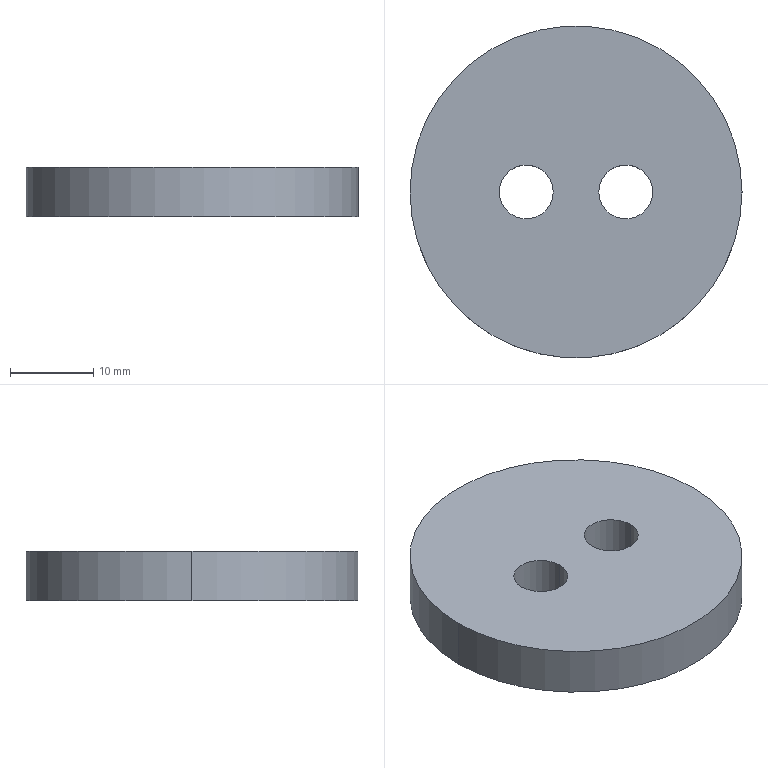Part | SolidWorks | features Extrusion 1 | 1 solid | 8 faces | box 40 x 40 x 6 mm | volume 7142 mm3 | cylinder 6 | plane 2 | commonest cylinder face diameters 6.5 x4 40 x2
STEP:
#1=CARTESIAN_POINT('',(-9.25,0.,6.));
#2=VERTEX_POINT('',#1);
#3=CARTESIAN_POINT('',(-2.75,0.,6.));
#4=VERTEX_POINT('',#3);
#5=CARTESIAN_POINT('',(-6.,0.,6.));
#6=DIRECTION('',(0.,0.,1.));
#7=DIRECTION('',(1.,0.,0.));
#8=AXIS2_PLACEMENT_3D('',#5,#6,#7);
#9=CIRCLE('',#8,3.25);
#10=EDGE_CURVE('',#2,#4,#9,.T.);
#11=ORIENTED_EDGE('',*,*,#10,.T.);
#12=CARTESIAN_POINT('',(-2.75,0.,0.));
#13=VERTEX_POINT('',#12);
#14=CARTESIAN_POINT('',(-2.75,0.,6.));
#15=DIRECTION('',(0.,0.,-1.));
#16=VECTOR('',#15,1000.);
#17=LINE('',#14,#16);
#18=EDGE_CURVE('',#4,#13,#17,.T.);
#19=ORIENTED_EDGE('',*,*,#18,.T.);
#20=CARTESIAN_POINT('',(-9.25,0.,0.));
#21=VERTEX_POINT('',#20);
#22=CARTESIAN_POINT('',(-6.,0.,0.));
#23=DIRECTION('',(0.,0.,1.));
#24=DIRECTION('',(1.,0.,0.));
#25=AXIS2_PLACEMENT_3D('',#22,#23,#24);
#26=CIRCLE('',#25,3.25);
#27=EDGE_CURVE('',#21,#13,#26,.T.);
#28=ORIENTED_EDGE('',*,*,#27,.F.);
#29=CARTESIAN_POINT('',(-9.25,0.,6.));
#30=DIRECTION('',(0.,0.,-1.));
#31=VECTOR('',#30,1000.);
#32=LINE('',#29,#31);
#33=EDGE_CURVE('',#2,#21,#32,.T.);
#34=ORIENTED_EDGE('',*,*,#33,.F.);
#35=EDGE_LOOP('',(#11,#19,#28,#34));
#36=FACE_OUTER_BOUND('',#35,.T.);
#37=CARTESIAN_POINT('',(-6.,0.,6.));
#38=DIRECTION('',(0.,0.,-1.));
#39=DIRECTION('',(-1.,0.,0.));
#40=AXIS2_PLACEMENT_3D('',#37,#38,#39);
#41=CYLINDRICAL_SURFACE('',#40,3.25);
#42=ADVANCED_FACE('',(#36),#41,.F.);
#43=CARTESIAN_POINT('',(2.75,0.,6.));
#44=VERTEX_POINT('',#43);
#45=CARTESIAN_POINT('',(9.25,0.,6.));
#46=VERTEX_POINT('',#45);
#47=CARTESIAN_POINT('',(6.,0.,6.));
#48=DIRECTION('',(0.,0.,1.));
#49=DIRECTION('',(1.,0.,0.));
#50=AXIS2_PLACEMENT_3D('',#47,#48,#49);
#51=CIRCLE('',#50,3.25);
#52=EDGE_CURVE('',#44,#46,#51,.T.);
#53=ORIENTED_EDGE('',*,*,#52,.T.);
#54=CARTESIAN_POINT('',(9.25,0.,0.));
#55=VERTEX_POINT('',#54);
#56=CARTESIAN_POINT('',(9.25,0.,6.));
#57=DIRECTION('',(0.,0.,-1.));
#58=VECTOR('',#57,1000.);
#59=LINE('',#56,#58);
#60=EDGE_CURVE('',#46,#55,#59,.T.);
#61=ORIENTED_EDGE('',*,*,#60,.T.);
#62=CARTESIAN_POINT('',(2.75,0.,0.));
#63=VERTEX_POINT('',#62);
#64=CARTESIAN_POINT('',(6.,0.,0.));
#65=DIRECTION('',(0.,0.,1.));
#66=DIRECTION('',(1.,0.,0.));
#67=AXIS2_PLACEMENT_3D('',#64,#65,#66);
#68=CIRCLE('',#67,3.25);
#69=EDGE_CURVE('',#63,#55,#68,.T.);
#70=ORIENTED_EDGE('',*,*,#69,.F.);
#71=CARTESIAN_POINT('',(2.75,0.,6.));
#72=DIRECTION('',(0.,0.,-1.));
#73=VECTOR('',#72,1000.);
#74=LINE('',#71,#73);
#75=EDGE_CURVE('',#44,#63,#74,.T.);
#76=ORIENTED_EDGE('',*,*,#75,.F.);
#77=EDGE_LOOP('',(#53,#61,#70,#76));
#78=FACE_OUTER_BOUND('',#77,.T.);
#79=CARTESIAN_POINT('',(6.,0.,6.));
#80=DIRECTION('',(0.,0.,-1.));
#81=DIRECTION('',(-1.,0.,0.));
#82=AXIS2_PLACEMENT_3D('',#79,#80,#81);
#83=CYLINDRICAL_SURFACE('',#82,3.25);
#84=ADVANCED_FACE('',(#78),#83,.F.);
#85=CARTESIAN_POINT('',(20.,0.,6.));
#86=VERTEX_POINT('',#85);
#87=CARTESIAN_POINT('',(-20.,0.,6.));
#88=VERTEX_POINT('',#87);
#89=CARTESIAN_POINT('',(0.,0.,6.));
#90=DIRECTION('',(0.,0.,1.));
#91=DIRECTION('',(1.,0.,0.));
#92=AXIS2_PLACEMENT_3D('',#89,#90,#91);
#93=CIRCLE('',#92,20.);
#94=EDGE_CURVE('',#86,#88,#93,.T.);
#95=ORIENTED_EDGE('',*,*,#94,.F.);
#96=CARTESIAN_POINT('',(20.,0.,0.));
#97=VERTEX_POINT('',#96);
#98=CARTESIAN_POINT('',(20.,0.,6.));
#99=DIRECTION('',(0.,0.,-1.));
#100=VECTOR('',#99,1000.);
#101=LINE('',#98,#100);
#102=EDGE_CURVE('',#86,#97,#101,.T.);
#103=ORIENTED_EDGE('',*,*,#102,.T.);
#104=CARTESIAN_POINT('',(-20.,0.,0.));
#105=VERTEX_POINT('',#104);
#106=CARTESIAN_POINT('',(0.,0.,0.));
#107=DIRECTION('',(0.,0.,1.));
#108=DIRECTION('',(1.,0.,0.));
#109=AXIS2_PLACEMENT_3D('',#106,#107,#108);
#110=CIRCLE('',#109,20.);
#111=EDGE_CURVE('',#97,#105,#110,.T.);
#112=ORIENTED_EDGE('',*,*,#111,.T.);
#113=CARTESIAN_POINT('',(-20.,0.,6.));
#114=DIRECTION('',(0.,0.,-1.));
#115=VECTOR('',#114,1000.);
#116=LINE('',#113,#115);
#117=EDGE_CURVE('',#88,#105,#116,.T.);
#118=ORIENTED_EDGE('',*,*,#117,.F.);
#119=EDGE_LOOP('',(#95,#103,#112,#118));
#120=FACE_OUTER_BOUND('',#119,.T.);
#121=CARTESIAN_POINT('',(0.,0.,6.));
#122=DIRECTION('',(0.,0.,-1.));
#123=DIRECTION('',(-1.,0.,0.));
#124=AXIS2_PLACEMENT_3D('',#121,#122,#123);
#125=CYLINDRICAL_SURFACE('',#124,20.);
#126=ADVANCED_FACE('',(#120),#125,.T.);
#127=ORIENTED_EDGE('',*,*,#52,.F.);
#128=CARTESIAN_POINT('',(6.,0.,6.));
#129=DIRECTION('',(0.,0.,1.));
#130=DIRECTION('',(1.,0.,0.));
#131=AXIS2_PLACEMENT_3D('',#128,#129,#130);
#132=CIRCLE('',#131,3.25);
#133=EDGE_CURVE('',#46,#44,#132,.T.);
#134=ORIENTED_EDGE('',*,*,#133,.F.);
#135=EDGE_LOOP('',(#127,#134));
#136=FACE_BOUND('',#135,.T.);
#137=CARTESIAN_POINT('',(0.,0.,6.));
#138=DIRECTION('',(0.,0.,1.));
#139=DIRECTION('',(1.,0.,0.));
#140=AXIS2_PLACEMENT_3D('',#137,#138,#139);
#141=CIRCLE('',#140,20.);
#142=EDGE_CURVE('',#88,#86,#141,.T.);
#143=ORIENTED_EDGE('',*,*,#142,.T.);
#144=ORIENTED_EDGE('',*,*,#94,.T.);
#145=EDGE_LOOP('',(#143,#144));
#146=FACE_OUTER_BOUND('',#145,.T.);
#147=ORIENTED_EDGE('',*,*,#10,.F.);
#148=CARTESIAN_POINT('',(-6.,0.,6.));
#149=DIRECTION('',(0.,0.,1.));
#150=DIRECTION('',(1.,0.,0.));
#151=AXIS2_PLACEMENT_3D('',#148,#149,#150);
#152=CIRCLE('',#151,3.25);
#153=EDGE_CURVE('',#4,#2,#152,.T.);
#154=ORIENTED_EDGE('',*,*,#153,.F.);
#155=EDGE_LOOP('',(#147,#154));
#156=FACE_BOUND('',#155,.T.);
#157=CARTESIAN_POINT('',(0.,0.,6.));
#158=DIRECTION('',(0.,0.,1.));
#159=DIRECTION('',(1.,0.,0.));
#160=AXIS2_PLACEMENT_3D('',#157,#158,#159);
#161=PLANE('',#160);
#162=ADVANCED_FACE('',(#136,#146,#156),#161,.T.);
#163=ORIENTED_EDGE('',*,*,#69,.T.);
#164=CARTESIAN_POINT('',(6.,0.,0.));
#165=DIRECTION('',(0.,0.,1.));
#166=DIRECTION('',(1.,0.,0.));
#167=AXIS2_PLACEMENT_3D('',#164,#165,#166);
#168=CIRCLE('',#167,3.25);
#169=EDGE_CURVE('',#55,#63,#168,.T.);
#170=ORIENTED_EDGE('',*,*,#169,.T.);
#171=EDGE_LOOP('',(#163,#170));
#172=FACE_BOUND('',#171,.T.);
#173=CARTESIAN_POINT('',(0.,0.,0.));
#174=DIRECTION('',(0.,0.,1.));
#175=DIRECTION('',(1.,0.,0.));
#176=AXIS2_PLACEMENT_3D('',#173,#174,#175);
#177=CIRCLE('',#176,20.);
#178=EDGE_CURVE('',#105,#97,#177,.T.);
#179=ORIENTED_EDGE('',*,*,#178,.F.);
#180=ORIENTED_EDGE('',*,*,#111,.F.);
#181=EDGE_LOOP('',(#179,#180));
#182=FACE_OUTER_BOUND('',#181,.T.);
#183=ORIENTED_EDGE('',*,*,#27,.T.);
#184=CARTESIAN_POINT('',(-6.,0.,0.));
#185=DIRECTION('',(0.,0.,1.));
#186=DIRECTION('',(1.,0.,0.));
#187=AXIS2_PLACEMENT_3D('',#184,#185,#186);
#188=CIRCLE('',#187,3.25);
#189=EDGE_CURVE('',#13,#21,#188,.T.);
#190=ORIENTED_EDGE('',*,*,#189,.T.);
#191=EDGE_LOOP('',(#183,#190));
#192=FACE_BOUND('',#191,.T.);
#193=CARTESIAN_POINT('',(0.,0.,0.));
#194=DIRECTION('',(0.,0.,1.));
#195=DIRECTION('',(1.,0.,0.));
#196=AXIS2_PLACEMENT_3D('',#193,#194,#195);
#197=PLANE('',#196);
#198=ADVANCED_FACE('',(#172,#182,#192),#197,.F.);
#199=ORIENTED_EDGE('',*,*,#102,.F.);
#200=ORIENTED_EDGE('',*,*,#142,.F.);
#201=ORIENTED_EDGE('',*,*,#117,.T.);
#202=ORIENTED_EDGE('',*,*,#178,.T.);
#203=EDGE_LOOP('',(#199,#200,#201,#202));
#204=FACE_OUTER_BOUND('',#203,.T.);
#205=CARTESIAN_POINT('',(0.,0.,6.));
#206=DIRECTION('',(0.,0.,-1.));
#207=DIRECTION('',(-1.,0.,0.));
#208=AXIS2_PLACEMENT_3D('',#205,#206,#207);
#209=CYLINDRICAL_SURFACE('',#208,20.);
#210=ADVANCED_FACE('',(#204),#209,.T.);
#211=ORIENTED_EDGE('',*,*,#60,.F.);
#212=ORIENTED_EDGE('',*,*,#133,.T.);
#213=ORIENTED_EDGE('',*,*,#75,.T.);
#214=ORIENTED_EDGE('',*,*,#169,.F.);
#215=EDGE_LOOP('',(#211,#212,#213,#214));
#216=FACE_OUTER_BOUND('',#215,.T.);
#217=CARTESIAN_POINT('',(6.,0.,6.));
#218=DIRECTION('',(0.,0.,-1.));
#219=DIRECTION('',(-1.,0.,0.));
#220=AXIS2_PLACEMENT_3D('',#217,#218,#219);
#221=CYLINDRICAL_SURFACE('',#220,3.25);
#222=ADVANCED_FACE('',(#216),#221,.F.);
#223=ORIENTED_EDGE('',*,*,#18,.F.);
#224=ORIENTED_EDGE('',*,*,#153,.T.);
#225=ORIENTED_EDGE('',*,*,#33,.T.);
#226=ORIENTED_EDGE('',*,*,#189,.F.);
#227=EDGE_LOOP('',(#223,#224,#225,#226));
#228=FACE_OUTER_BOUND('',#227,.T.);
#229=CARTESIAN_POINT('',(-6.,0.,6.));
#230=DIRECTION('',(0.,0.,-1.));
#231=DIRECTION('',(-1.,0.,0.));
#232=AXIS2_PLACEMENT_3D('',#229,#230,#231);
#233=CYLINDRICAL_SURFACE('',#232,3.25);
#234=ADVANCED_FACE('',(#228),#233,.F.);
#235=CLOSED_SHELL('',(#42,#84,#126,#162,#198,#210,#222,#234));
#236=MANIFOLD_SOLID_BREP('',#235);
#237=CARTESIAN_POINT('',(0.,0.,0.));
#238=DIRECTION('',(0.,0.,1.));
#239=DIRECTION('',(1.,0.,0.));
#240=AXIS2_PLACEMENT_3D('',#237,#238,#239);
#241=(LENGTH_UNIT()NAMED_UNIT(*)SI_UNIT(.MILLI.,.METRE.));
#242=UNCERTAINTY_MEASURE_WITH_UNIT(LENGTH_MEASURE(0.00001),#241,'','');
#243=(NAMED_UNIT(*)PLANE_ANGLE_UNIT()SI_UNIT($,.RADIAN.));
#244=(NAMED_UNIT(*)SI_UNIT($,.STERADIAN.)SOLID_ANGLE_UNIT());
#245=(GEOMETRIC_REPRESENTATION_CONTEXT(3)GLOBAL_UNCERTAINTY_ASSIGNED_CONTEXT((#242))GLOBAL_UNIT_ASSIGNED_CONTEXT((#241,#243,#244))REPRESENTATION_CONTEXT('',''));
#246=ADVANCED_BREP_SHAPE_REPRESENTATION('',(#236,#240),#245);